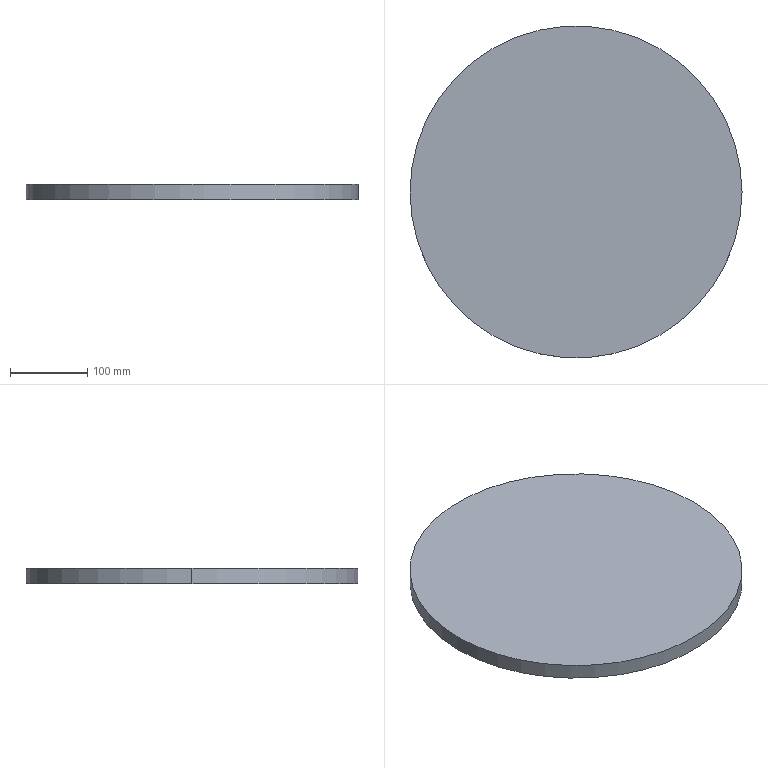Part | SolidWorks | features Extrusion 1 | 1 solid | 4 faces | box 430 x 430 x 20 mm | volume 2904402 mm3 | cylinder 2 | plane 2 | commonest cylinder face diameters 430 x2
STEP:
#1=CARTESIAN_POINT('',(215.,0.,20.));
#2=VERTEX_POINT('',#1);
#3=CARTESIAN_POINT('',(-215.,0.,20.));
#4=VERTEX_POINT('',#3);
#5=CARTESIAN_POINT('',(0.,0.,20.));
#6=DIRECTION('',(0.,0.,1.));
#7=DIRECTION('',(1.,0.,0.));
#8=AXIS2_PLACEMENT_3D('',#5,#6,#7);
#9=CIRCLE('',#8,215.);
#10=EDGE_CURVE('',#2,#4,#9,.T.);
#11=ORIENTED_EDGE('',*,*,#10,.F.);
#12=CARTESIAN_POINT('',(215.,0.,0.));
#13=VERTEX_POINT('',#12);
#14=CARTESIAN_POINT('',(215.,0.,20.));
#15=DIRECTION('',(0.,0.,-1.));
#16=VECTOR('',#15,1000.);
#17=LINE('',#14,#16);
#18=EDGE_CURVE('',#2,#13,#17,.T.);
#19=ORIENTED_EDGE('',*,*,#18,.T.);
#20=CARTESIAN_POINT('',(-215.,0.,0.));
#21=VERTEX_POINT('',#20);
#22=CARTESIAN_POINT('',(0.,0.,0.));
#23=DIRECTION('',(0.,0.,1.));
#24=DIRECTION('',(1.,0.,0.));
#25=AXIS2_PLACEMENT_3D('',#22,#23,#24);
#26=CIRCLE('',#25,215.);
#27=EDGE_CURVE('',#13,#21,#26,.T.);
#28=ORIENTED_EDGE('',*,*,#27,.T.);
#29=CARTESIAN_POINT('',(-215.,0.,20.));
#30=DIRECTION('',(0.,0.,-1.));
#31=VECTOR('',#30,1000.);
#32=LINE('',#29,#31);
#33=EDGE_CURVE('',#4,#21,#32,.T.);
#34=ORIENTED_EDGE('',*,*,#33,.F.);
#35=EDGE_LOOP('',(#11,#19,#28,#34));
#36=FACE_OUTER_BOUND('',#35,.T.);
#37=CARTESIAN_POINT('',(0.,0.,20.));
#38=DIRECTION('',(0.,0.,-1.));
#39=DIRECTION('',(-1.,0.,0.));
#40=AXIS2_PLACEMENT_3D('',#37,#38,#39);
#41=CYLINDRICAL_SURFACE('',#40,215.);
#42=ADVANCED_FACE('',(#36),#41,.T.);
#43=ORIENTED_EDGE('',*,*,#18,.F.);
#44=CARTESIAN_POINT('',(0.,0.,20.));
#45=DIRECTION('',(0.,0.,1.));
#46=DIRECTION('',(1.,0.,0.));
#47=AXIS2_PLACEMENT_3D('',#44,#45,#46);
#48=CIRCLE('',#47,215.);
#49=EDGE_CURVE('',#4,#2,#48,.T.);
#50=ORIENTED_EDGE('',*,*,#49,.F.);
#51=ORIENTED_EDGE('',*,*,#33,.T.);
#52=CARTESIAN_POINT('',(0.,0.,0.));
#53=DIRECTION('',(0.,0.,1.));
#54=DIRECTION('',(1.,0.,0.));
#55=AXIS2_PLACEMENT_3D('',#52,#53,#54);
#56=CIRCLE('',#55,215.);
#57=EDGE_CURVE('',#21,#13,#56,.T.);
#58=ORIENTED_EDGE('',*,*,#57,.T.);
#59=EDGE_LOOP('',(#43,#50,#51,#58));
#60=FACE_OUTER_BOUND('',#59,.T.);
#61=CARTESIAN_POINT('',(0.,0.,20.));
#62=DIRECTION('',(0.,0.,-1.));
#63=DIRECTION('',(-1.,0.,0.));
#64=AXIS2_PLACEMENT_3D('',#61,#62,#63);
#65=CYLINDRICAL_SURFACE('',#64,215.);
#66=ADVANCED_FACE('',(#60),#65,.T.);
#67=ORIENTED_EDGE('',*,*,#49,.T.);
#68=ORIENTED_EDGE('',*,*,#10,.T.);
#69=EDGE_LOOP('',(#67,#68));
#70=FACE_OUTER_BOUND('',#69,.T.);
#71=CARTESIAN_POINT('',(0.,0.,20.));
#72=DIRECTION('',(0.,0.,1.));
#73=DIRECTION('',(1.,0.,0.));
#74=AXIS2_PLACEMENT_3D('',#71,#72,#73);
#75=PLANE('',#74);
#76=ADVANCED_FACE('',(#70),#75,.T.);
#77=ORIENTED_EDGE('',*,*,#57,.F.);
#78=ORIENTED_EDGE('',*,*,#27,.F.);
#79=EDGE_LOOP('',(#77,#78));
#80=FACE_OUTER_BOUND('',#79,.T.);
#81=CARTESIAN_POINT('',(0.,0.,0.));
#82=DIRECTION('',(0.,0.,1.));
#83=DIRECTION('',(1.,0.,0.));
#84=AXIS2_PLACEMENT_3D('',#81,#82,#83);
#85=PLANE('',#84);
#86=ADVANCED_FACE('',(#80),#85,.F.);
#87=CLOSED_SHELL('',(#42,#66,#76,#86));
#88=MANIFOLD_SOLID_BREP('',#87);
#89=CARTESIAN_POINT('',(0.,0.,0.));
#90=DIRECTION('',(0.,0.,1.));
#91=DIRECTION('',(1.,0.,0.));
#92=AXIS2_PLACEMENT_3D('',#89,#90,#91);
#93=(LENGTH_UNIT()NAMED_UNIT(*)SI_UNIT(.MILLI.,.METRE.));
#94=UNCERTAINTY_MEASURE_WITH_UNIT(LENGTH_MEASURE(0.00001),#93,'','');
#95=(NAMED_UNIT(*)PLANE_ANGLE_UNIT()SI_UNIT($,.RADIAN.));
#96=(NAMED_UNIT(*)SI_UNIT($,.STERADIAN.)SOLID_ANGLE_UNIT());
#97=(GEOMETRIC_REPRESENTATION_CONTEXT(3)GLOBAL_UNCERTAINTY_ASSIGNED_CONTEXT((#94))GLOBAL_UNIT_ASSIGNED_CONTEXT((#93,#95,#96))REPRESENTATION_CONTEXT('',''));
#98=ADVANCED_BREP_SHAPE_REPRESENTATION('',(#88,#92),#97);